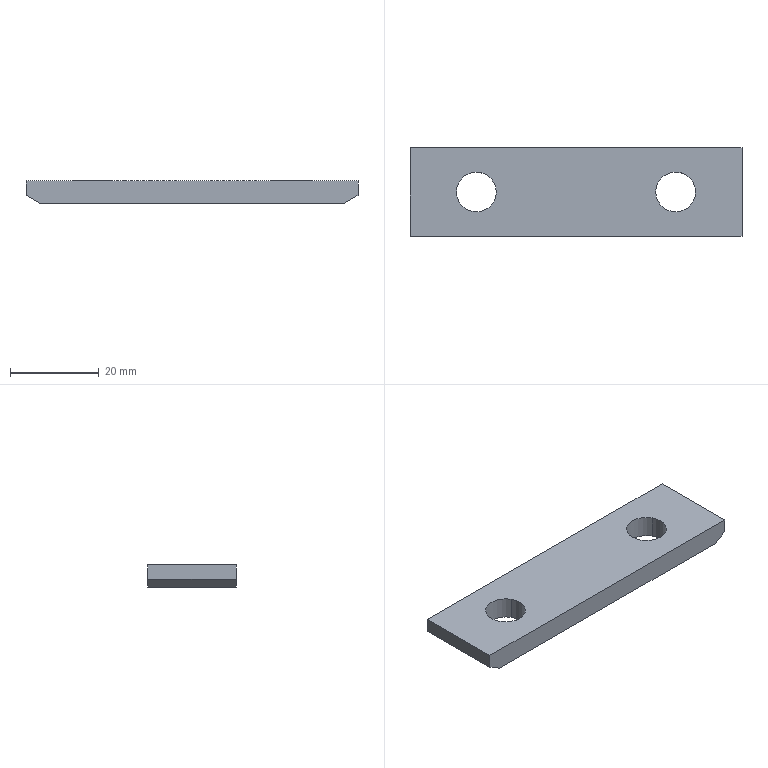Part | CATIA | 1 solid | 12 faces | box 75 x 20 x 5 mm | volume 6760 mm3 | plane 8 | cylinder 4 | commonest cylinder face diameters 9 x4
STEP:
#1=CARTESIAN_POINT('',(-37.5,-17.,1.732));
#2=VERTEX_POINT('',#1);
#3=CARTESIAN_POINT('',(-37.5,-17.,5.));
#4=VERTEX_POINT('',#3);
#5=CARTESIAN_POINT('',(-37.5,-17.,3.366));
#6=DIRECTION('',(0.,0.,1.));
#7=VECTOR('',#6,1.);
#8=LINE('',#5,#7);
#9=EDGE_CURVE('',#2,#4,#8,.T.);
#10=ORIENTED_EDGE('',*,*,#9,.T.);
#11=CARTESIAN_POINT('',(-37.5,3.,5.));
#12=VERTEX_POINT('',#11);
#13=CARTESIAN_POINT('',(-37.5,-7.,5.));
#14=DIRECTION('',(0.,-1.,0.));
#15=VECTOR('',#14,1.);
#16=LINE('',#13,#15);
#17=EDGE_CURVE('',#12,#4,#16,.T.);
#18=ORIENTED_EDGE('',*,*,#17,.F.);
#19=CARTESIAN_POINT('',(-37.5,3.,1.732));
#20=VERTEX_POINT('',#19);
#21=CARTESIAN_POINT('',(-37.5,3.,3.366));
#22=DIRECTION('',(0.,0.,1.));
#23=VECTOR('',#22,1.);
#24=LINE('',#21,#23);
#25=EDGE_CURVE('',#20,#12,#24,.T.);
#26=ORIENTED_EDGE('',*,*,#25,.F.);
#27=CARTESIAN_POINT('',(-37.5,-7.,1.732));
#28=DIRECTION('',(0.,-1.,0.));
#29=VECTOR('',#28,1.);
#30=LINE('',#27,#29);
#31=EDGE_CURVE('',#20,#2,#30,.T.);
#32=ORIENTED_EDGE('',*,*,#31,.T.);
#33=EDGE_LOOP('',(#10,#18,#26,#32));
#34=FACE_OUTER_BOUND('',#33,.T.);
#35=CARTESIAN_POINT('',(-37.5,3.,0.));
#36=DIRECTION('',(-1.,0.,0.));
#37=DIRECTION('',(0.,-1.,0.));
#38=AXIS2_PLACEMENT_3D('',#35,#36,#37);
#39=PLANE('',#38);
#40=ADVANCED_FACE('',(#34),#39,.T.);
#41=CARTESIAN_POINT('',(-34.5,-17.,0.));
#42=VERTEX_POINT('',#41);
#43=CARTESIAN_POINT('',(-36.,-17.,0.866));
#44=DIRECTION('',(-0.866,0.,0.5));
#45=VECTOR('',#44,1.);
#46=LINE('',#43,#45);
#47=EDGE_CURVE('',#42,#2,#46,.T.);
#48=ORIENTED_EDGE('',*,*,#47,.T.);
#49=ORIENTED_EDGE('',*,*,#31,.F.);
#50=CARTESIAN_POINT('',(-34.5,3.,0.));
#51=VERTEX_POINT('',#50);
#52=CARTESIAN_POINT('',(-36.,3.,0.866));
#53=DIRECTION('',(-0.866,0.,0.5));
#54=VECTOR('',#53,1.);
#55=LINE('',#52,#54);
#56=EDGE_CURVE('',#20,#51,#55,.F.);
#57=ORIENTED_EDGE('',*,*,#56,.T.);
#58=CARTESIAN_POINT('',(-34.5,-7.,0.));
#59=DIRECTION('',(0.,-1.,0.));
#60=VECTOR('',#59,1.);
#61=LINE('',#58,#60);
#62=EDGE_CURVE('',#51,#42,#61,.T.);
#63=ORIENTED_EDGE('',*,*,#62,.T.);
#64=EDGE_LOOP('',(#48,#49,#57,#63));
#65=FACE_OUTER_BOUND('',#64,.T.);
#66=CARTESIAN_POINT('',(-34.5,7.,0.));
#67=DIRECTION('',(-0.5,0.,-0.866));
#68=DIRECTION('',(0.,-1.,0.));
#69=AXIS2_PLACEMENT_3D('',#66,#67,#68);
#70=PLANE('',#69);
#71=ADVANCED_FACE('',(#65),#70,.T.);
#72=CARTESIAN_POINT('',(37.5,3.,1.732));
#73=VERTEX_POINT('',#72);
#74=CARTESIAN_POINT('',(37.5,3.,5.));
#75=VERTEX_POINT('',#74);
#76=CARTESIAN_POINT('',(37.5,3.,3.366));
#77=DIRECTION('',(0.,0.,1.));
#78=VECTOR('',#77,1.);
#79=LINE('',#76,#78);
#80=EDGE_CURVE('',#73,#75,#79,.T.);
#81=ORIENTED_EDGE('',*,*,#80,.T.);
#82=CARTESIAN_POINT('',(37.5,-17.,5.));
#83=VERTEX_POINT('',#82);
#84=CARTESIAN_POINT('',(37.5,-7.,5.));
#85=DIRECTION('',(0.,1.,0.));
#86=VECTOR('',#85,1.);
#87=LINE('',#84,#86);
#88=EDGE_CURVE('',#83,#75,#87,.T.);
#89=ORIENTED_EDGE('',*,*,#88,.F.);
#90=CARTESIAN_POINT('',(37.5,-17.,1.732));
#91=VERTEX_POINT('',#90);
#92=CARTESIAN_POINT('',(37.5,-17.,3.366));
#93=DIRECTION('',(0.,0.,1.));
#94=VECTOR('',#93,1.);
#95=LINE('',#92,#94);
#96=EDGE_CURVE('',#91,#83,#95,.T.);
#97=ORIENTED_EDGE('',*,*,#96,.F.);
#98=CARTESIAN_POINT('',(37.5,-7.,1.732));
#99=DIRECTION('',(0.,1.,0.));
#100=VECTOR('',#99,1.);
#101=LINE('',#98,#100);
#102=EDGE_CURVE('',#91,#73,#101,.T.);
#103=ORIENTED_EDGE('',*,*,#102,.T.);
#104=EDGE_LOOP('',(#81,#89,#97,#103));
#105=FACE_OUTER_BOUND('',#104,.T.);
#106=CARTESIAN_POINT('',(37.5,-17.,0.));
#107=DIRECTION('',(1.,0.,0.));
#108=DIRECTION('',(0.,1.,0.));
#109=AXIS2_PLACEMENT_3D('',#106,#107,#108);
#110=PLANE('',#109);
#111=ADVANCED_FACE('',(#105),#110,.T.);
#112=ORIENTED_EDGE('',*,*,#96,.T.);
#113=CARTESIAN_POINT('',(0.,-17.,5.));
#114=DIRECTION('',(1.,0.,0.));
#115=VECTOR('',#114,1.);
#116=LINE('',#113,#115);
#117=EDGE_CURVE('',#4,#83,#116,.T.);
#118=ORIENTED_EDGE('',*,*,#117,.F.);
#119=ORIENTED_EDGE('',*,*,#9,.F.);
#120=ORIENTED_EDGE('',*,*,#47,.F.);
#121=CARTESIAN_POINT('',(34.5,-17.,0.));
#122=VERTEX_POINT('',#121);
#123=CARTESIAN_POINT('',(0.,-17.,0.));
#124=DIRECTION('',(1.,0.,0.));
#125=VECTOR('',#124,1.);
#126=LINE('',#123,#125);
#127=EDGE_CURVE('',#42,#122,#126,.T.);
#128=ORIENTED_EDGE('',*,*,#127,.T.);
#129=CARTESIAN_POINT('',(36.,-17.,0.866));
#130=DIRECTION('',(-0.866,0.,-0.5));
#131=VECTOR('',#130,1.);
#132=LINE('',#129,#131);
#133=EDGE_CURVE('',#91,#122,#132,.T.);
#134=ORIENTED_EDGE('',*,*,#133,.F.);
#135=EDGE_LOOP('',(#112,#118,#119,#120,#128,#134));
#136=FACE_OUTER_BOUND('',#135,.T.);
#137=CARTESIAN_POINT('',(-37.5,-17.,0.));
#138=DIRECTION('',(0.,-1.,0.));
#139=DIRECTION('',(1.,0.,0.));
#140=AXIS2_PLACEMENT_3D('',#137,#138,#139);
#141=PLANE('',#140);
#142=ADVANCED_FACE('',(#136),#141,.T.);
#143=CARTESIAN_POINT('',(34.5,3.,0.));
#144=VERTEX_POINT('',#143);
#145=CARTESIAN_POINT('',(0.,3.,0.));
#146=DIRECTION('',(-1.,0.,0.));
#147=VECTOR('',#146,1.);
#148=LINE('',#145,#147);
#149=EDGE_CURVE('',#144,#51,#148,.T.);
#150=ORIENTED_EDGE('',*,*,#149,.T.);
#151=ORIENTED_EDGE('',*,*,#56,.F.);
#152=ORIENTED_EDGE('',*,*,#25,.T.);
#153=CARTESIAN_POINT('',(0.,3.,5.));
#154=DIRECTION('',(-1.,0.,0.));
#155=VECTOR('',#154,1.);
#156=LINE('',#153,#155);
#157=EDGE_CURVE('',#75,#12,#156,.T.);
#158=ORIENTED_EDGE('',*,*,#157,.F.);
#159=ORIENTED_EDGE('',*,*,#80,.F.);
#160=CARTESIAN_POINT('',(36.,3.,0.866));
#161=DIRECTION('',(-0.866,0.,-0.5));
#162=VECTOR('',#161,1.);
#163=LINE('',#160,#162);
#164=EDGE_CURVE('',#144,#73,#163,.F.);
#165=ORIENTED_EDGE('',*,*,#164,.F.);
#166=EDGE_LOOP('',(#150,#151,#152,#158,#159,#165));
#167=FACE_OUTER_BOUND('',#166,.T.);
#168=CARTESIAN_POINT('',(37.5,3.,0.));
#169=DIRECTION('',(0.,1.,0.));
#170=DIRECTION('',(-1.,0.,0.));
#171=AXIS2_PLACEMENT_3D('',#168,#169,#170);
#172=PLANE('',#171);
#173=ADVANCED_FACE('',(#167),#172,.T.);
#174=ORIENTED_EDGE('',*,*,#164,.T.);
#175=ORIENTED_EDGE('',*,*,#102,.F.);
#176=ORIENTED_EDGE('',*,*,#133,.T.);
#177=CARTESIAN_POINT('',(34.5,-7.,0.));
#178=DIRECTION('',(0.,1.,0.));
#179=VECTOR('',#178,1.);
#180=LINE('',#177,#179);
#181=EDGE_CURVE('',#122,#144,#180,.T.);
#182=ORIENTED_EDGE('',*,*,#181,.T.);
#183=EDGE_LOOP('',(#174,#175,#176,#182));
#184=FACE_OUTER_BOUND('',#183,.T.);
#185=CARTESIAN_POINT('',(34.5,-21.,0.));
#186=DIRECTION('',(0.5,0.,-0.866));
#187=DIRECTION('',(0.,1.,0.));
#188=AXIS2_PLACEMENT_3D('',#185,#186,#187);
#189=PLANE('',#188);
#190=ADVANCED_FACE('',(#184),#189,.T.);
#191=ORIENTED_EDGE('',*,*,#181,.F.);
#192=ORIENTED_EDGE('',*,*,#127,.F.);
#193=ORIENTED_EDGE('',*,*,#62,.F.);
#194=ORIENTED_EDGE('',*,*,#149,.F.);
#195=EDGE_LOOP('',(#191,#192,#193,#194));
#196=FACE_OUTER_BOUND('',#195,.T.);
#197=CARTESIAN_POINT('',(-18.551,-4.843,0.));
#198=VERTEX_POINT('',#197);
#199=CARTESIAN_POINT('',(-26.449,-9.157,0.));
#200=VERTEX_POINT('',#199);
#201=CARTESIAN_POINT('',(-22.5,-7.,0.));
#202=DIRECTION('',(0.,0.,1.));
#203=AXIS2_PLACEMENT_3D('',#201,#202,$);
#204=CIRCLE('',#203,4.5);
#205=EDGE_CURVE('',#198,#200,#204,.T.);
#206=ORIENTED_EDGE('',*,*,#205,.T.);
#207=CARTESIAN_POINT('',(-22.5,-7.,0.));
#208=DIRECTION('',(0.,0.,1.));
#209=AXIS2_PLACEMENT_3D('',#207,#208,$);
#210=CIRCLE('',#209,4.5);
#211=EDGE_CURVE('',#200,#198,#210,.T.);
#212=ORIENTED_EDGE('',*,*,#211,.T.);
#213=EDGE_LOOP('',(#206,#212));
#214=FACE_BOUND('',#213,.T.);
#215=CARTESIAN_POINT('',(26.449,-4.843,0.));
#216=VERTEX_POINT('',#215);
#217=CARTESIAN_POINT('',(18.551,-9.157,0.));
#218=VERTEX_POINT('',#217);
#219=CARTESIAN_POINT('',(22.5,-7.,0.));
#220=DIRECTION('',(0.,0.,1.));
#221=AXIS2_PLACEMENT_3D('',#219,#220,$);
#222=CIRCLE('',#221,4.5);
#223=EDGE_CURVE('',#216,#218,#222,.T.);
#224=ORIENTED_EDGE('',*,*,#223,.T.);
#225=CARTESIAN_POINT('',(22.5,-7.,0.));
#226=DIRECTION('',(0.,0.,1.));
#227=AXIS2_PLACEMENT_3D('',#225,#226,$);
#228=CIRCLE('',#227,4.5);
#229=EDGE_CURVE('',#218,#216,#228,.T.);
#230=ORIENTED_EDGE('',*,*,#229,.T.);
#231=EDGE_LOOP('',(#224,#230));
#232=FACE_BOUND('',#231,.T.);
#233=CARTESIAN_POINT('',(0.,0.,0.));
#234=DIRECTION('',(0.,0.,1.));
#235=DIRECTION('',(1.,0.,0.));
#236=AXIS2_PLACEMENT_3D('',#233,#234,#235);
#237=PLANE('',#236);
#238=ADVANCED_FACE('',(#196,#214,#232),#237,.F.);
#239=ORIENTED_EDGE('',*,*,#117,.T.);
#240=ORIENTED_EDGE('',*,*,#88,.T.);
#241=ORIENTED_EDGE('',*,*,#157,.T.);
#242=ORIENTED_EDGE('',*,*,#17,.T.);
#243=EDGE_LOOP('',(#239,#240,#241,#242));
#244=FACE_OUTER_BOUND('',#243,.T.);
#245=CARTESIAN_POINT('',(-18.551,-4.843,5.));
#246=VERTEX_POINT('',#245);
#247=CARTESIAN_POINT('',(-26.449,-9.157,5.));
#248=VERTEX_POINT('',#247);
#249=CARTESIAN_POINT('',(-22.5,-7.,5.));
#250=DIRECTION('',(0.,0.,1.));
#251=AXIS2_PLACEMENT_3D('',#249,#250,$);
#252=CIRCLE('',#251,4.5);
#253=EDGE_CURVE('',#246,#248,#252,.T.);
#254=ORIENTED_EDGE('',*,*,#253,.F.);
#255=CARTESIAN_POINT('',(-22.5,-7.,5.));
#256=DIRECTION('',(0.,0.,1.));
#257=AXIS2_PLACEMENT_3D('',#255,#256,$);
#258=CIRCLE('',#257,4.5);
#259=EDGE_CURVE('',#248,#246,#258,.T.);
#260=ORIENTED_EDGE('',*,*,#259,.F.);
#261=EDGE_LOOP('',(#254,#260));
#262=FACE_BOUND('',#261,.T.);
#263=CARTESIAN_POINT('',(26.449,-4.843,5.));
#264=VERTEX_POINT('',#263);
#265=CARTESIAN_POINT('',(18.551,-9.157,5.));
#266=VERTEX_POINT('',#265);
#267=CARTESIAN_POINT('',(22.5,-7.,5.));
#268=DIRECTION('',(0.,0.,1.));
#269=AXIS2_PLACEMENT_3D('',#267,#268,$);
#270=CIRCLE('',#269,4.5);
#271=EDGE_CURVE('',#264,#266,#270,.T.);
#272=ORIENTED_EDGE('',*,*,#271,.F.);
#273=CARTESIAN_POINT('',(22.5,-7.,5.));
#274=DIRECTION('',(0.,0.,1.));
#275=AXIS2_PLACEMENT_3D('',#273,#274,$);
#276=CIRCLE('',#275,4.5);
#277=EDGE_CURVE('',#266,#264,#276,.T.);
#278=ORIENTED_EDGE('',*,*,#277,.F.);
#279=EDGE_LOOP('',(#272,#278));
#280=FACE_BOUND('',#279,.T.);
#281=CARTESIAN_POINT('',(0.,0.,5.));
#282=DIRECTION('',(0.,0.,1.));
#283=DIRECTION('',(1.,0.,0.));
#284=AXIS2_PLACEMENT_3D('',#281,#282,#283);
#285=PLANE('',#284);
#286=ADVANCED_FACE('',(#244,#262,#280),#285,.T.);
#287=ORIENTED_EDGE('',*,*,#277,.T.);
#288=CARTESIAN_POINT('',(26.449,-4.843,11.8));
#289=DIRECTION('',(0.,0.,1.));
#290=VECTOR('',#289,1.);
#291=LINE('',#288,#290);
#292=EDGE_CURVE('',#264,#216,#291,.F.);
#293=ORIENTED_EDGE('',*,*,#292,.T.);
#294=ORIENTED_EDGE('',*,*,#229,.F.);
#295=CARTESIAN_POINT('',(18.551,-9.157,11.8));
#296=DIRECTION('',(0.,0.,1.));
#297=VECTOR('',#296,1.);
#298=LINE('',#295,#297);
#299=EDGE_CURVE('',#266,#218,#298,.F.);
#300=ORIENTED_EDGE('',*,*,#299,.F.);
#301=EDGE_LOOP('',(#287,#293,#294,#300));
#302=FACE_OUTER_BOUND('',#301,.T.);
#303=CARTESIAN_POINT('',(22.5,-7.,0.1));
#304=DIRECTION('',(0.,0.,1.));
#305=DIRECTION('',(0.8776,0.4794,0.));
#306=AXIS2_PLACEMENT_3D('',#303,#304,#305);
#307=CYLINDRICAL_SURFACE('',#306,4.5);
#308=ADVANCED_FACE('',(#302),#307,.F.);
#309=ORIENTED_EDGE('',*,*,#271,.T.);
#310=ORIENTED_EDGE('',*,*,#299,.T.);
#311=ORIENTED_EDGE('',*,*,#223,.F.);
#312=ORIENTED_EDGE('',*,*,#292,.F.);
#313=EDGE_LOOP('',(#309,#310,#311,#312));
#314=FACE_OUTER_BOUND('',#313,.T.);
#315=ADVANCED_FACE('',(#314),#307,.F.);
#316=ORIENTED_EDGE('',*,*,#259,.T.);
#317=CARTESIAN_POINT('',(-18.551,-4.843,11.8));
#318=DIRECTION('',(0.,0.,1.));
#319=VECTOR('',#318,1.);
#320=LINE('',#317,#319);
#321=EDGE_CURVE('',#246,#198,#320,.F.);
#322=ORIENTED_EDGE('',*,*,#321,.T.);
#323=ORIENTED_EDGE('',*,*,#211,.F.);
#324=CARTESIAN_POINT('',(-26.449,-9.157,11.8));
#325=DIRECTION('',(0.,0.,1.));
#326=VECTOR('',#325,1.);
#327=LINE('',#324,#326);
#328=EDGE_CURVE('',#248,#200,#327,.F.);
#329=ORIENTED_EDGE('',*,*,#328,.F.);
#330=EDGE_LOOP('',(#316,#322,#323,#329));
#331=FACE_OUTER_BOUND('',#330,.T.);
#332=CARTESIAN_POINT('',(-22.5,-7.,0.1));
#333=DIRECTION('',(0.,0.,1.));
#334=DIRECTION('',(0.8776,0.4794,0.));
#335=AXIS2_PLACEMENT_3D('',#332,#333,#334);
#336=CYLINDRICAL_SURFACE('',#335,4.5);
#337=ADVANCED_FACE('',(#331),#336,.F.);
#338=ORIENTED_EDGE('',*,*,#253,.T.);
#339=ORIENTED_EDGE('',*,*,#328,.T.);
#340=ORIENTED_EDGE('',*,*,#205,.F.);
#341=ORIENTED_EDGE('',*,*,#321,.F.);
#342=EDGE_LOOP('',(#338,#339,#340,#341));
#343=FACE_OUTER_BOUND('',#342,.T.);
#344=ADVANCED_FACE('',(#343),#336,.F.);
#345=CLOSED_SHELL('',(#40,#71,#111,#142,#173,#190,#238,#286,#308,#315,#337,#344));
#346=MANIFOLD_SOLID_BREP('',#345);
#347=(LENGTH_UNIT()NAMED_UNIT(*)SI_UNIT(.MILLI.,.METRE.));
#348=UNCERTAINTY_MEASURE_WITH_UNIT(LENGTH_MEASURE(0.005),#347,'','');
#349=(NAMED_UNIT(*)PLANE_ANGLE_UNIT()SI_UNIT($,.RADIAN.));
#350=(NAMED_UNIT(*)SI_UNIT($,.STERADIAN.)SOLID_ANGLE_UNIT());
#351=(GEOMETRIC_REPRESENTATION_CONTEXT(3)GLOBAL_UNCERTAINTY_ASSIGNED_CONTEXT((#348))GLOBAL_UNIT_ASSIGNED_CONTEXT((#347,#349,#350))REPRESENTATION_CONTEXT('',''));
#352=ADVANCED_BREP_SHAPE_REPRESENTATION('',(#346),#351);